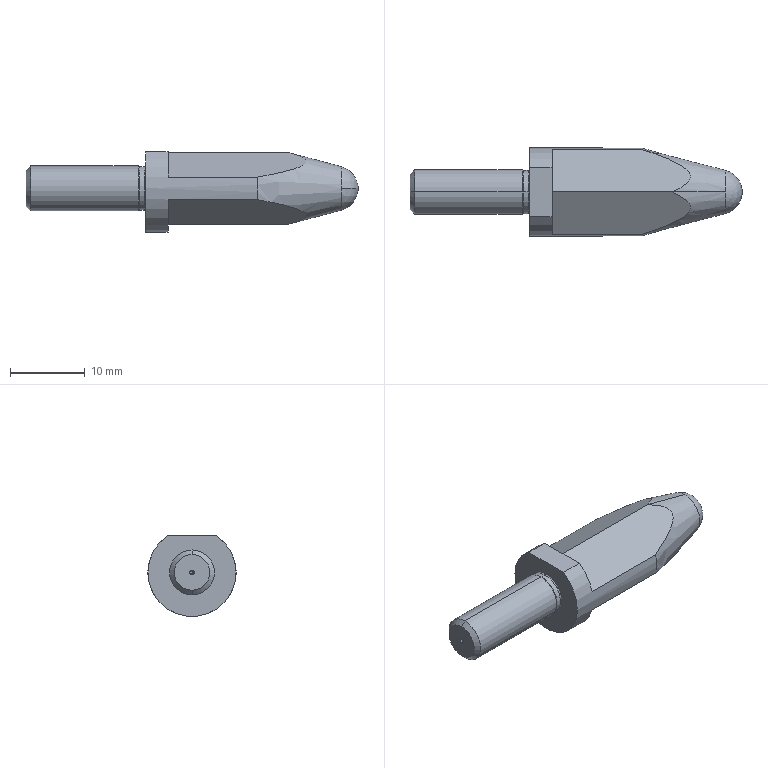Part | STEP file | FLNND6_P11_8_B15_0_L10_FLNND6-P11.8-B15.0-L10 | 1 solid | 28 faces | box 44.415 x 11.8 x 10.8 mm | volume 2279 mm3 | plane 9 | cone 8 | cylinder 5 | torus 4 | sphere 2 | commonest cylinder face diameters 5.8 x2 6 x2 11.8 x1